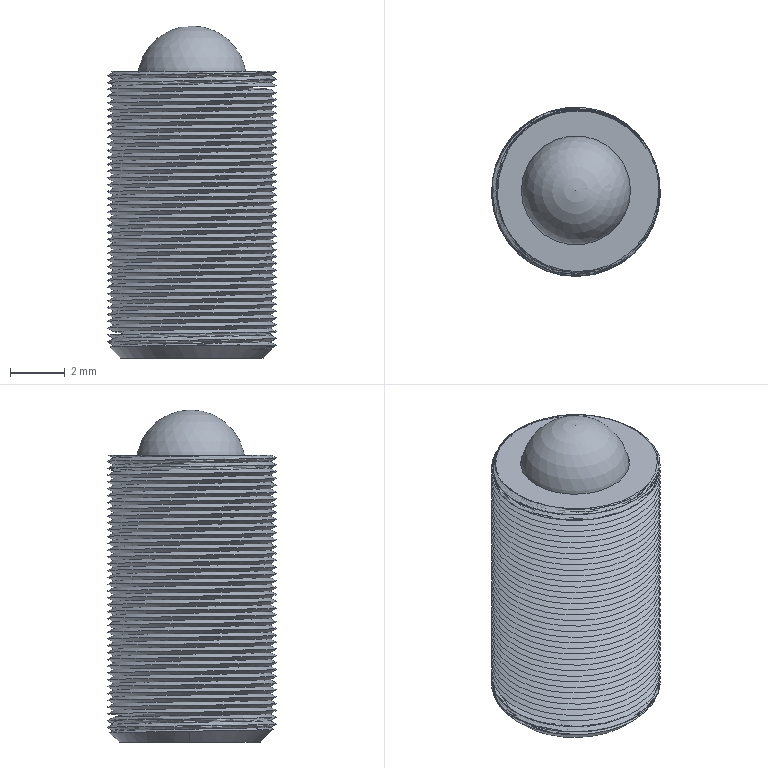Part | SolidWorks | 2 solids | 20 faces | box 6.183 x 6.183 x 12.162 mm | volume 269.276 mm3 | plane 9 | cone 5 | cylinder 2 | spline 2 | sphere 2 | commonest cylinder face diameters 4 x2